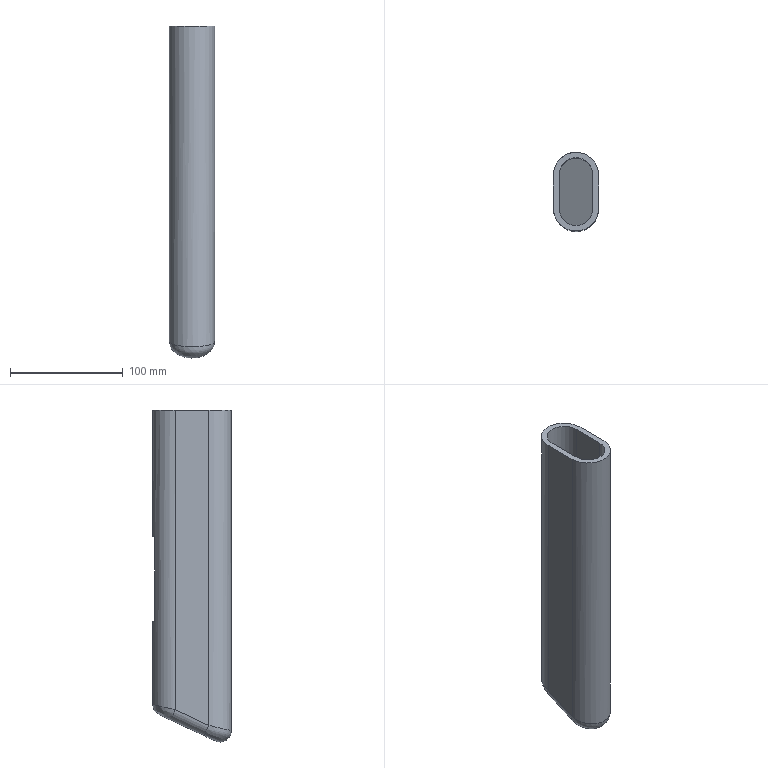Part | STEP file | Part 6 | 1 solid | 19 faces | box 40 x 70 x 294.303 mm | volume 238300 mm3 | plane 11 | cylinder 6 | spline 2 | commonest cylinder face diameters 20 x2 30 x2 40 x2